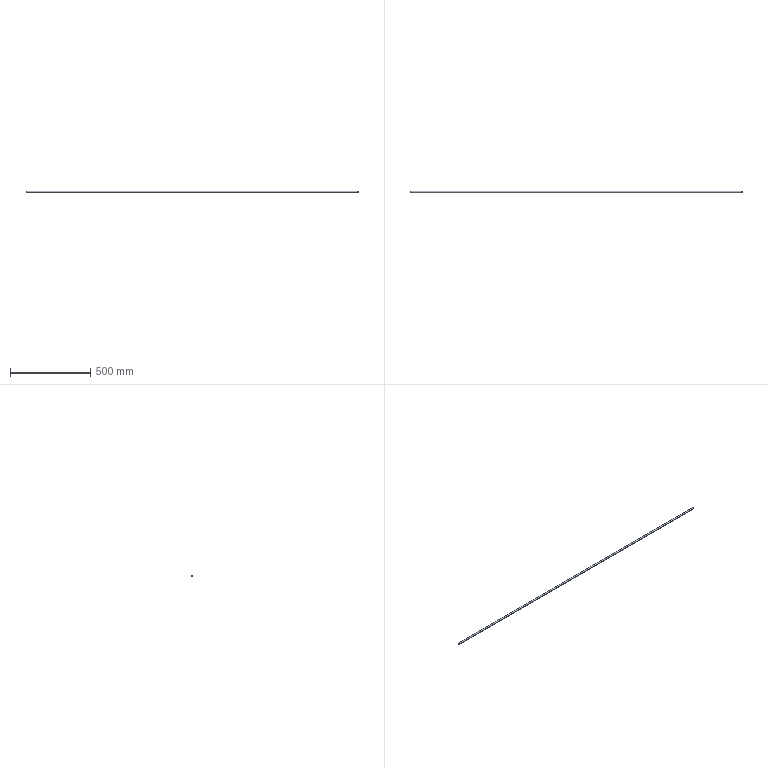Part | NX | features BREP 1 | 1 solid | 8 faces | box 2064 x 9.525 x 9.525 mm | volume 147037 mm3 | cone 4 | plane 2 | cylinder 2 | commonest cylinder face diameters 9.525 x2
STEP:
#1=CARTESIAN_POINT('',(-1031.875,3.975,0.));
#2=VERTEX_POINT('',#1);
#3=CARTESIAN_POINT('',(-1031.875,-3.975,0.));
#4=VERTEX_POINT('',#3);
#5=CARTESIAN_POINT('',(-1031.875,0.,0.));
#6=DIRECTION('',(1.,0.,0.));
#7=DIRECTION('',(0.,1.,0.));
#8=AXIS2_PLACEMENT_3D('',#5,#6,#7);
#9=CIRCLE('',#8,3.975);
#10=EDGE_CURVE('',#2,#4,#9,.T.);
#11=ORIENTED_EDGE('',*,*,#10,.F.);
#12=CARTESIAN_POINT('',(-1031.875,0.,0.));
#13=DIRECTION('',(1.,0.,0.));
#14=DIRECTION('',(0.,-1.,0.));
#15=AXIS2_PLACEMENT_3D('',#12,#13,#14);
#16=CIRCLE('',#15,3.975);
#17=EDGE_CURVE('',#4,#2,#16,.T.);
#18=ORIENTED_EDGE('',*,*,#17,.F.);
#19=EDGE_LOOP('',(#11,#18));
#20=FACE_BOUND('',#19,.T.);
#21=CARTESIAN_POINT('',(-1031.875,0.,0.));
#22=DIRECTION('',(1.,0.,0.));
#23=DIRECTION('',(0.,1.,0.));
#24=AXIS2_PLACEMENT_3D('',#21,#22,#23);
#25=PLANE('',#24);
#26=ADVANCED_FACE('',(#20),#25,.F.);
#27=CARTESIAN_POINT('',(-1031.088,4.763,0.));
#28=VERTEX_POINT('',#27);
#29=CARTESIAN_POINT('',(-1031.875,3.975,0.));
#30=DIRECTION('',(0.7071,0.7071,0.));
#31=VECTOR('',#30,1000.);
#32=LINE('',#29,#31);
#33=EDGE_CURVE('',#28,#2,#32,.F.);
#34=ORIENTED_EDGE('',*,*,#33,.F.);
#35=CARTESIAN_POINT('',(-1031.088,-4.763,0.));
#36=VERTEX_POINT('',#35);
#37=CARTESIAN_POINT('',(-1031.088,0.,0.));
#38=DIRECTION('',(1.,0.,0.));
#39=DIRECTION('',(0.,-1.,0.));
#40=AXIS2_PLACEMENT_3D('',#37,#38,#39);
#41=CIRCLE('',#40,4.763);
#42=EDGE_CURVE('',#36,#28,#41,.T.);
#43=ORIENTED_EDGE('',*,*,#42,.F.);
#44=CARTESIAN_POINT('',(-1031.875,-3.975,0.));
#45=DIRECTION('',(0.7071,-0.7071,0.));
#46=VECTOR('',#45,1000.);
#47=LINE('',#44,#46);
#48=EDGE_CURVE('',#36,#4,#47,.F.);
#49=ORIENTED_EDGE('',*,*,#48,.T.);
#50=ORIENTED_EDGE('',*,*,#17,.T.);
#51=EDGE_LOOP('',(#34,#43,#49,#50));
#52=FACE_BOUND('',#51,.T.);
#53=CARTESIAN_POINT('',(-1031.481,0.,0.));
#54=DIRECTION('',(1.,0.,0.));
#55=DIRECTION('',(0.,-1.,0.));
#56=AXIS2_PLACEMENT_3D('',#53,#54,#55);
#57=CONICAL_SURFACE('',#56,4.369,0.7854);
#58=ADVANCED_FACE('',(#52),#57,.T.);
#59=ORIENTED_EDGE('',*,*,#48,.F.);
#60=CARTESIAN_POINT('',(-1031.088,0.,0.));
#61=DIRECTION('',(1.,0.,0.));
#62=DIRECTION('',(0.,1.,0.));
#63=AXIS2_PLACEMENT_3D('',#60,#61,#62);
#64=CIRCLE('',#63,4.763);
#65=EDGE_CURVE('',#28,#36,#64,.T.);
#66=ORIENTED_EDGE('',*,*,#65,.F.);
#67=ORIENTED_EDGE('',*,*,#33,.T.);
#68=ORIENTED_EDGE('',*,*,#10,.T.);
#69=EDGE_LOOP('',(#59,#66,#67,#68));
#70=FACE_BOUND('',#69,.T.);
#71=CARTESIAN_POINT('',(-1031.481,0.,0.));
#72=DIRECTION('',(1.,0.,0.));
#73=DIRECTION('',(0.,-1.,0.));
#74=AXIS2_PLACEMENT_3D('',#71,#72,#73);
#75=CONICAL_SURFACE('',#74,4.369,0.7854);
#76=ADVANCED_FACE('',(#70),#75,.T.);
#77=CARTESIAN_POINT('',(1031.088,-4.763,0.));
#78=VERTEX_POINT('',#77);
#79=CARTESIAN_POINT('',(-1031.088,-4.763,0.));
#80=DIRECTION('',(1.,0.,0.));
#81=VECTOR('',#80,1000.);
#82=LINE('',#79,#81);
#83=EDGE_CURVE('',#36,#78,#82,.T.);
#84=ORIENTED_EDGE('',*,*,#83,.T.);
#85=CARTESIAN_POINT('',(1031.088,4.763,0.));
#86=VERTEX_POINT('',#85);
#87=CARTESIAN_POINT('',(1031.088,0.,0.));
#88=DIRECTION('',(1.,0.,0.));
#89=DIRECTION('',(0.,1.,0.));
#90=AXIS2_PLACEMENT_3D('',#87,#88,#89);
#91=CIRCLE('',#90,4.763);
#92=EDGE_CURVE('',#86,#78,#91,.T.);
#93=ORIENTED_EDGE('',*,*,#92,.F.);
#94=CARTESIAN_POINT('',(-1031.088,4.763,0.));
#95=DIRECTION('',(1.,0.,0.));
#96=VECTOR('',#95,1000.);
#97=LINE('',#94,#96);
#98=EDGE_CURVE('',#28,#86,#97,.T.);
#99=ORIENTED_EDGE('',*,*,#98,.F.);
#100=ORIENTED_EDGE('',*,*,#65,.T.);
#101=EDGE_LOOP('',(#84,#93,#99,#100));
#102=FACE_BOUND('',#101,.T.);
#103=CARTESIAN_POINT('',(-1031.875,0.,0.));
#104=DIRECTION('',(1.,0.,0.));
#105=DIRECTION('',(0.,-1.,0.));
#106=AXIS2_PLACEMENT_3D('',#103,#104,#105);
#107=CYLINDRICAL_SURFACE('',#106,4.763);
#108=ADVANCED_FACE('',(#102),#107,.T.);
#109=ORIENTED_EDGE('',*,*,#98,.T.);
#110=CARTESIAN_POINT('',(1031.088,0.,0.));
#111=DIRECTION('',(1.,0.,0.));
#112=DIRECTION('',(0.,-1.,0.));
#113=AXIS2_PLACEMENT_3D('',#110,#111,#112);
#114=CIRCLE('',#113,4.763);
#115=EDGE_CURVE('',#78,#86,#114,.T.);
#116=ORIENTED_EDGE('',*,*,#115,.F.);
#117=ORIENTED_EDGE('',*,*,#83,.F.);
#118=ORIENTED_EDGE('',*,*,#42,.T.);
#119=EDGE_LOOP('',(#109,#116,#117,#118));
#120=FACE_BOUND('',#119,.T.);
#121=CARTESIAN_POINT('',(-1031.875,0.,0.));
#122=DIRECTION('',(1.,0.,0.));
#123=DIRECTION('',(0.,-1.,0.));
#124=AXIS2_PLACEMENT_3D('',#121,#122,#123);
#125=CYLINDRICAL_SURFACE('',#124,4.763);
#126=ADVANCED_FACE('',(#120),#125,.T.);
#127=CARTESIAN_POINT('',(1031.875,-3.975,0.));
#128=VERTEX_POINT('',#127);
#129=CARTESIAN_POINT('',(1031.875,-3.975,0.));
#130=DIRECTION('',(-0.7071,-0.7071,0.));
#131=VECTOR('',#130,1000.);
#132=LINE('',#129,#131);
#133=EDGE_CURVE('',#128,#78,#132,.T.);
#134=ORIENTED_EDGE('',*,*,#133,.T.);
#135=ORIENTED_EDGE('',*,*,#115,.T.);
#136=CARTESIAN_POINT('',(1031.875,3.975,0.));
#137=VERTEX_POINT('',#136);
#138=CARTESIAN_POINT('',(1031.875,3.975,0.));
#139=DIRECTION('',(-0.7071,0.7071,0.));
#140=VECTOR('',#139,1000.);
#141=LINE('',#138,#140);
#142=EDGE_CURVE('',#137,#86,#141,.T.);
#143=ORIENTED_EDGE('',*,*,#142,.F.);
#144=CARTESIAN_POINT('',(1031.875,0.,0.));
#145=DIRECTION('',(1.,0.,0.));
#146=DIRECTION('',(0.,-1.,0.));
#147=AXIS2_PLACEMENT_3D('',#144,#145,#146);
#148=CIRCLE('',#147,3.975);
#149=EDGE_CURVE('',#128,#137,#148,.T.);
#150=ORIENTED_EDGE('',*,*,#149,.F.);
#151=EDGE_LOOP('',(#134,#135,#143,#150));
#152=FACE_BOUND('',#151,.T.);
#153=CARTESIAN_POINT('',(1031.481,0.,0.));
#154=DIRECTION('',(-1.,0.,0.));
#155=DIRECTION('',(0.,1.,0.));
#156=AXIS2_PLACEMENT_3D('',#153,#154,#155);
#157=CONICAL_SURFACE('',#156,4.369,0.7854);
#158=ADVANCED_FACE('',(#152),#157,.T.);
#159=CARTESIAN_POINT('',(1031.875,0.,0.));
#160=DIRECTION('',(1.,0.,0.));
#161=DIRECTION('',(0.,1.,0.));
#162=AXIS2_PLACEMENT_3D('',#159,#160,#161);
#163=CIRCLE('',#162,3.975);
#164=EDGE_CURVE('',#137,#128,#163,.T.);
#165=ORIENTED_EDGE('',*,*,#164,.T.);
#166=ORIENTED_EDGE('',*,*,#149,.T.);
#167=EDGE_LOOP('',(#165,#166));
#168=FACE_BOUND('',#167,.T.);
#169=CARTESIAN_POINT('',(1031.875,0.,0.));
#170=DIRECTION('',(1.,0.,0.));
#171=DIRECTION('',(0.,1.,0.));
#172=AXIS2_PLACEMENT_3D('',#169,#170,#171);
#173=PLANE('',#172);
#174=ADVANCED_FACE('',(#168),#173,.T.);
#175=ORIENTED_EDGE('',*,*,#142,.T.);
#176=ORIENTED_EDGE('',*,*,#92,.T.);
#177=ORIENTED_EDGE('',*,*,#133,.F.);
#178=ORIENTED_EDGE('',*,*,#164,.F.);
#179=EDGE_LOOP('',(#175,#176,#177,#178));
#180=FACE_BOUND('',#179,.T.);
#181=CARTESIAN_POINT('',(1031.481,0.,0.));
#182=DIRECTION('',(-1.,0.,0.));
#183=DIRECTION('',(0.,1.,0.));
#184=AXIS2_PLACEMENT_3D('',#181,#182,#183);
#185=CONICAL_SURFACE('',#184,4.369,0.7854);
#186=ADVANCED_FACE('',(#180),#185,.T.);
#187=CLOSED_SHELL('',(#26,#58,#76,#108,#126,#158,#174,#186));
#188=MANIFOLD_SOLID_BREP('',#187);
#189=(LENGTH_UNIT()NAMED_UNIT(*)SI_UNIT(.MILLI.,.METRE.));
#190=UNCERTAINTY_MEASURE_WITH_UNIT(LENGTH_MEASURE(0.00001),#189,'','');
#191=(NAMED_UNIT(*)PLANE_ANGLE_UNIT()SI_UNIT($,.RADIAN.));
#192=(NAMED_UNIT(*)SI_UNIT($,.STERADIAN.)SOLID_ANGLE_UNIT());
#193=(GEOMETRIC_REPRESENTATION_CONTEXT(3)GLOBAL_UNCERTAINTY_ASSIGNED_CONTEXT((#190))GLOBAL_UNIT_ASSIGNED_CONTEXT((#189,#191,#192))REPRESENTATION_CONTEXT('',''));
#194=ADVANCED_BREP_SHAPE_REPRESENTATION('',(#188),#193);